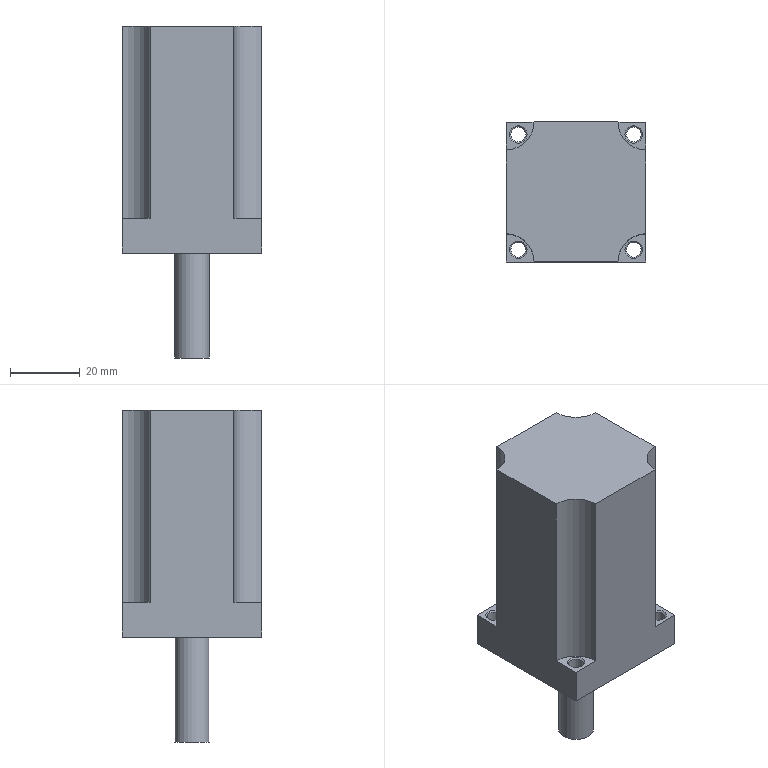Part | NX | features DATUM_CSYS 5, EXTRUDE 4, SIMPLE HOLE 4, SKETCH 4, SYMBOLIC_THREAD 4, HOLE PACKAGE 1 | 2 solids | 31 faces | box 40 x 40 x 95 mm | volume 97876 mm3 | plane 13 | cylinder 10 | cone 8 | commonest cylinder face diameters 4.2 x4 16 x4 10 x2
STEP:
#1=CARTESIAN_POINT('',(-14.,16.5,10.));
#2=VERTEX_POINT('',#1);
#3=CARTESIAN_POINT('',(-16.5,16.5,10.));
#4=DIRECTION('',(0.,0.,1.));
#5=DIRECTION('',(1.,0.,0.));
#6=AXIS2_PLACEMENT_3D('',#3,#4,#5);
#7=CIRCLE('',#6,2.5);
#8=EDGE_CURVE('',#2,#2,#7,.F.);
#9=ORIENTED_EDGE('',*,*,#8,.T.);
#10=EDGE_LOOP('',(#9));
#11=FACE_BOUND('',#10,.T.);
#12=CARTESIAN_POINT('',(-12.,20.,10.));
#13=VERTEX_POINT('',#12);
#14=CARTESIAN_POINT('',(-20.,12.,10.));
#15=VERTEX_POINT('',#14);
#16=CARTESIAN_POINT('',(-20.,20.,10.));
#17=DIRECTION('',(0.,0.,-1.));
#18=DIRECTION('',(0.,1.,0.));
#19=AXIS2_PLACEMENT_3D('',#16,#17,#18);
#20=CIRCLE('',#19,8.);
#21=EDGE_CURVE('',#13,#15,#20,.T.);
#22=ORIENTED_EDGE('',*,*,#21,.F.);
#23=CARTESIAN_POINT('',(-20.,20.,10.));
#24=VERTEX_POINT('',#23);
#25=CARTESIAN_POINT('',(20.,20.,10.));
#26=DIRECTION('',(-1.,0.,0.));
#27=VECTOR('',#26,1000.);
#28=LINE('',#25,#27);
#29=EDGE_CURVE('',#13,#24,#28,.T.);
#30=ORIENTED_EDGE('',*,*,#29,.T.);
#31=CARTESIAN_POINT('',(-20.,20.,10.));
#32=DIRECTION('',(0.,-1.,0.));
#33=VECTOR('',#32,1000.);
#34=LINE('',#31,#33);
#35=EDGE_CURVE('',#24,#15,#34,.T.);
#36=ORIENTED_EDGE('',*,*,#35,.T.);
#37=EDGE_LOOP('',(#22,#30,#36));
#38=FACE_BOUND('',#37,.T.);
#39=CARTESIAN_POINT('',(0.,0.,10.));
#40=DIRECTION('',(0.,0.,1.));
#41=DIRECTION('',(1.,0.,0.));
#42=AXIS2_PLACEMENT_3D('',#39,#40,#41);
#43=PLANE('',#42);
#44=ADVANCED_FACE('',(#11,#38),#43,.T.);
#45=CARTESIAN_POINT('',(19.,16.5,10.));
#46=VERTEX_POINT('',#45);
#47=CARTESIAN_POINT('',(16.5,16.5,10.));
#48=DIRECTION('',(0.,0.,1.));
#49=DIRECTION('',(1.,0.,0.));
#50=AXIS2_PLACEMENT_3D('',#47,#48,#49);
#51=CIRCLE('',#50,2.5);
#52=EDGE_CURVE('',#46,#46,#51,.F.);
#53=ORIENTED_EDGE('',*,*,#52,.T.);
#54=EDGE_LOOP('',(#53));
#55=FACE_BOUND('',#54,.T.);
#56=CARTESIAN_POINT('',(20.,12.,10.));
#57=VERTEX_POINT('',#56);
#58=CARTESIAN_POINT('',(12.,20.,10.));
#59=VERTEX_POINT('',#58);
#60=CARTESIAN_POINT('',(20.,20.,10.));
#61=DIRECTION('',(0.,0.,-1.));
#62=DIRECTION('',(0.,1.,0.));
#63=AXIS2_PLACEMENT_3D('',#60,#61,#62);
#64=CIRCLE('',#63,8.);
#65=EDGE_CURVE('',#57,#59,#64,.T.);
#66=ORIENTED_EDGE('',*,*,#65,.F.);
#67=CARTESIAN_POINT('',(20.,20.,10.));
#68=VERTEX_POINT('',#67);
#69=CARTESIAN_POINT('',(20.,-20.,10.));
#70=DIRECTION('',(0.,1.,0.));
#71=VECTOR('',#70,1000.);
#72=LINE('',#69,#71);
#73=EDGE_CURVE('',#57,#68,#72,.T.);
#74=ORIENTED_EDGE('',*,*,#73,.T.);
#75=CARTESIAN_POINT('',(20.,20.,10.));
#76=DIRECTION('',(-1.,0.,0.));
#77=VECTOR('',#76,1000.);
#78=LINE('',#75,#77);
#79=EDGE_CURVE('',#68,#59,#78,.T.);
#80=ORIENTED_EDGE('',*,*,#79,.T.);
#81=EDGE_LOOP('',(#66,#74,#80));
#82=FACE_BOUND('',#81,.T.);
#83=CARTESIAN_POINT('',(0.,0.,10.));
#84=DIRECTION('',(0.,0.,1.));
#85=DIRECTION('',(1.,0.,0.));
#86=AXIS2_PLACEMENT_3D('',#83,#84,#85);
#87=PLANE('',#86);
#88=ADVANCED_FACE('',(#55,#82),#87,.T.);
#89=CARTESIAN_POINT('',(19.,-16.5,10.));
#90=VERTEX_POINT('',#89);
#91=CARTESIAN_POINT('',(16.5,-16.5,10.));
#92=DIRECTION('',(0.,0.,1.));
#93=DIRECTION('',(1.,0.,0.));
#94=AXIS2_PLACEMENT_3D('',#91,#92,#93);
#95=CIRCLE('',#94,2.5);
#96=EDGE_CURVE('',#90,#90,#95,.F.);
#97=ORIENTED_EDGE('',*,*,#96,.T.);
#98=EDGE_LOOP('',(#97));
#99=FACE_BOUND('',#98,.T.);
#100=CARTESIAN_POINT('',(12.,-20.,10.));
#101=VERTEX_POINT('',#100);
#102=CARTESIAN_POINT('',(20.,-12.,10.));
#103=VERTEX_POINT('',#102);
#104=CARTESIAN_POINT('',(20.,-20.,10.));
#105=DIRECTION('',(0.,0.,-1.));
#106=DIRECTION('',(0.,-1.,0.));
#107=AXIS2_PLACEMENT_3D('',#104,#105,#106);
#108=CIRCLE('',#107,8.);
#109=EDGE_CURVE('',#101,#103,#108,.T.);
#110=ORIENTED_EDGE('',*,*,#109,.F.);
#111=CARTESIAN_POINT('',(20.,-20.,10.));
#112=VERTEX_POINT('',#111);
#113=CARTESIAN_POINT('',(-20.,-20.,10.));
#114=DIRECTION('',(1.,0.,0.));
#115=VECTOR('',#114,1000.);
#116=LINE('',#113,#115);
#117=EDGE_CURVE('',#101,#112,#116,.T.);
#118=ORIENTED_EDGE('',*,*,#117,.T.);
#119=CARTESIAN_POINT('',(20.,-20.,10.));
#120=DIRECTION('',(0.,1.,0.));
#121=VECTOR('',#120,1000.);
#122=LINE('',#119,#121);
#123=EDGE_CURVE('',#112,#103,#122,.T.);
#124=ORIENTED_EDGE('',*,*,#123,.T.);
#125=EDGE_LOOP('',(#110,#118,#124));
#126=FACE_BOUND('',#125,.T.);
#127=CARTESIAN_POINT('',(0.,0.,10.));
#128=DIRECTION('',(0.,0.,1.));
#129=DIRECTION('',(1.,0.,0.));
#130=AXIS2_PLACEMENT_3D('',#127,#128,#129);
#131=PLANE('',#130);
#132=ADVANCED_FACE('',(#99,#126),#131,.T.);
#133=CARTESIAN_POINT('',(-14.,-16.5,10.));
#134=VERTEX_POINT('',#133);
#135=CARTESIAN_POINT('',(-16.5,-16.5,10.));
#136=DIRECTION('',(0.,0.,1.));
#137=DIRECTION('',(1.,0.,0.));
#138=AXIS2_PLACEMENT_3D('',#135,#136,#137);
#139=CIRCLE('',#138,2.5);
#140=EDGE_CURVE('',#134,#134,#139,.F.);
#141=ORIENTED_EDGE('',*,*,#140,.T.);
#142=EDGE_LOOP('',(#141));
#143=FACE_BOUND('',#142,.T.);
#144=CARTESIAN_POINT('',(-20.,-12.,10.));
#145=VERTEX_POINT('',#144);
#146=CARTESIAN_POINT('',(-12.,-20.,10.));
#147=VERTEX_POINT('',#146);
#148=CARTESIAN_POINT('',(-20.,-20.,10.));
#149=DIRECTION('',(0.,0.,-1.));
#150=DIRECTION('',(0.,-1.,0.));
#151=AXIS2_PLACEMENT_3D('',#148,#149,#150);
#152=CIRCLE('',#151,8.);
#153=EDGE_CURVE('',#145,#147,#152,.T.);
#154=ORIENTED_EDGE('',*,*,#153,.F.);
#155=CARTESIAN_POINT('',(-20.,-20.,10.));
#156=VERTEX_POINT('',#155);
#157=CARTESIAN_POINT('',(-20.,20.,10.));
#158=DIRECTION('',(0.,-1.,0.));
#159=VECTOR('',#158,1000.);
#160=LINE('',#157,#159);
#161=EDGE_CURVE('',#145,#156,#160,.T.);
#162=ORIENTED_EDGE('',*,*,#161,.T.);
#163=CARTESIAN_POINT('',(-20.,-20.,10.));
#164=DIRECTION('',(1.,0.,0.));
#165=VECTOR('',#164,1000.);
#166=LINE('',#163,#165);
#167=EDGE_CURVE('',#156,#147,#166,.T.);
#168=ORIENTED_EDGE('',*,*,#167,.T.);
#169=EDGE_LOOP('',(#154,#162,#168));
#170=FACE_BOUND('',#169,.T.);
#171=CARTESIAN_POINT('',(0.,0.,10.));
#172=DIRECTION('',(0.,0.,1.));
#173=DIRECTION('',(1.,0.,0.));
#174=AXIS2_PLACEMENT_3D('',#171,#172,#173);
#175=PLANE('',#174);
#176=ADVANCED_FACE('',(#143,#170),#175,.T.);
#177=CARTESIAN_POINT('',(-20.,20.,0.));
#178=VERTEX_POINT('',#177);
#179=CARTESIAN_POINT('',(-20.,-20.,0.));
#180=VERTEX_POINT('',#179);
#181=CARTESIAN_POINT('',(-20.,20.,0.));
#182=DIRECTION('',(0.,-1.,0.));
#183=VECTOR('',#182,1000.);
#184=LINE('',#181,#183);
#185=EDGE_CURVE('',#178,#180,#184,.T.);
#186=ORIENTED_EDGE('',*,*,#185,.T.);
#187=CARTESIAN_POINT('',(-20.,-20.,10.));
#188=DIRECTION('',(0.,0.,-1.));
#189=VECTOR('',#188,1000.);
#190=LINE('',#187,#189);
#191=EDGE_CURVE('',#156,#180,#190,.T.);
#192=ORIENTED_EDGE('',*,*,#191,.F.);
#193=ORIENTED_EDGE('',*,*,#161,.F.);
#194=CARTESIAN_POINT('',(-20.,-12.,65.));
#195=VERTEX_POINT('',#194);
#196=CARTESIAN_POINT('',(-20.,-12.,65.));
#197=DIRECTION('',(0.,0.,-1.));
#198=VECTOR('',#197,1000.);
#199=LINE('',#196,#198);
#200=EDGE_CURVE('',#195,#145,#199,.T.);
#201=ORIENTED_EDGE('',*,*,#200,.F.);
#202=CARTESIAN_POINT('',(-20.,12.,65.));
#203=VERTEX_POINT('',#202);
#204=CARTESIAN_POINT('',(-20.,12.,65.));
#205=DIRECTION('',(0.,-1.,0.));
#206=VECTOR('',#205,1000.);
#207=LINE('',#204,#206);
#208=EDGE_CURVE('',#203,#195,#207,.T.);
#209=ORIENTED_EDGE('',*,*,#208,.F.);
#210=CARTESIAN_POINT('',(-20.,12.,65.));
#211=DIRECTION('',(0.,0.,-1.));
#212=VECTOR('',#211,1000.);
#213=LINE('',#210,#212);
#214=EDGE_CURVE('',#203,#15,#213,.T.);
#215=ORIENTED_EDGE('',*,*,#214,.T.);
#216=ORIENTED_EDGE('',*,*,#35,.F.);
#217=CARTESIAN_POINT('',(-20.,20.,10.));
#218=DIRECTION('',(0.,0.,-1.));
#219=VECTOR('',#218,1000.);
#220=LINE('',#217,#219);
#221=EDGE_CURVE('',#24,#178,#220,.T.);
#222=ORIENTED_EDGE('',*,*,#221,.T.);
#223=EDGE_LOOP('',(#186,#192,#193,#201,#209,#215,#216,#222));
#224=FACE_BOUND('',#223,.T.);
#225=CARTESIAN_POINT('',(-20.,20.,10.));
#226=DIRECTION('',(1.,0.,0.));
#227=DIRECTION('',(0.,0.,-1.));
#228=AXIS2_PLACEMENT_3D('',#225,#226,#227);
#229=PLANE('',#228);
#230=ADVANCED_FACE('',(#224),#229,.F.);
#231=CARTESIAN_POINT('',(20.,-20.,0.));
#232=VERTEX_POINT('',#231);
#233=CARTESIAN_POINT('',(-20.,-20.,0.));
#234=DIRECTION('',(1.,0.,0.));
#235=VECTOR('',#234,1000.);
#236=LINE('',#233,#235);
#237=EDGE_CURVE('',#180,#232,#236,.T.);
#238=ORIENTED_EDGE('',*,*,#237,.T.);
#239=CARTESIAN_POINT('',(20.,-20.,10.));
#240=DIRECTION('',(0.,0.,-1.));
#241=VECTOR('',#240,1000.);
#242=LINE('',#239,#241);
#243=EDGE_CURVE('',#112,#232,#242,.T.);
#244=ORIENTED_EDGE('',*,*,#243,.F.);
#245=ORIENTED_EDGE('',*,*,#117,.F.);
#246=CARTESIAN_POINT('',(12.,-20.,65.));
#247=VERTEX_POINT('',#246);
#248=CARTESIAN_POINT('',(12.,-20.,65.));
#249=DIRECTION('',(0.,0.,-1.));
#250=VECTOR('',#249,1000.);
#251=LINE('',#248,#250);
#252=EDGE_CURVE('',#247,#101,#251,.T.);
#253=ORIENTED_EDGE('',*,*,#252,.F.);
#254=CARTESIAN_POINT('',(-12.,-20.,65.));
#255=VERTEX_POINT('',#254);
#256=CARTESIAN_POINT('',(-12.,-20.,65.));
#257=DIRECTION('',(1.,0.,0.));
#258=VECTOR('',#257,1000.);
#259=LINE('',#256,#258);
#260=EDGE_CURVE('',#255,#247,#259,.T.);
#261=ORIENTED_EDGE('',*,*,#260,.F.);
#262=CARTESIAN_POINT('',(-12.,-20.,65.));
#263=DIRECTION('',(0.,0.,-1.));
#264=VECTOR('',#263,1000.);
#265=LINE('',#262,#264);
#266=EDGE_CURVE('',#255,#147,#265,.T.);
#267=ORIENTED_EDGE('',*,*,#266,.T.);
#268=ORIENTED_EDGE('',*,*,#167,.F.);
#269=ORIENTED_EDGE('',*,*,#191,.T.);
#270=EDGE_LOOP('',(#238,#244,#245,#253,#261,#267,#268,#269));
#271=FACE_BOUND('',#270,.T.);
#272=CARTESIAN_POINT('',(-20.,-20.,10.));
#273=DIRECTION('',(0.,1.,0.));
#274=DIRECTION('',(0.,0.,1.));
#275=AXIS2_PLACEMENT_3D('',#272,#273,#274);
#276=PLANE('',#275);
#277=ADVANCED_FACE('',(#271),#276,.F.);
#278=CARTESIAN_POINT('',(20.,20.,0.));
#279=VERTEX_POINT('',#278);
#280=CARTESIAN_POINT('',(20.,-20.,0.));
#281=DIRECTION('',(0.,1.,0.));
#282=VECTOR('',#281,1000.);
#283=LINE('',#280,#282);
#284=EDGE_CURVE('',#232,#279,#283,.T.);
#285=ORIENTED_EDGE('',*,*,#284,.T.);
#286=CARTESIAN_POINT('',(20.,20.,10.));
#287=DIRECTION('',(0.,0.,-1.));
#288=VECTOR('',#287,1000.);
#289=LINE('',#286,#288);
#290=EDGE_CURVE('',#68,#279,#289,.T.);
#291=ORIENTED_EDGE('',*,*,#290,.F.);
#292=ORIENTED_EDGE('',*,*,#73,.F.);
#293=CARTESIAN_POINT('',(20.,12.,65.));
#294=VERTEX_POINT('',#293);
#295=CARTESIAN_POINT('',(20.,12.,65.));
#296=DIRECTION('',(0.,0.,-1.));
#297=VECTOR('',#296,1000.);
#298=LINE('',#295,#297);
#299=EDGE_CURVE('',#294,#57,#298,.T.);
#300=ORIENTED_EDGE('',*,*,#299,.F.);
#301=CARTESIAN_POINT('',(20.,-12.,65.));
#302=VERTEX_POINT('',#301);
#303=CARTESIAN_POINT('',(20.,-12.,65.));
#304=DIRECTION('',(0.,1.,0.));
#305=VECTOR('',#304,1000.);
#306=LINE('',#303,#305);
#307=EDGE_CURVE('',#302,#294,#306,.T.);
#308=ORIENTED_EDGE('',*,*,#307,.F.);
#309=CARTESIAN_POINT('',(20.,-12.,65.));
#310=DIRECTION('',(0.,0.,-1.));
#311=VECTOR('',#310,1000.);
#312=LINE('',#309,#311);
#313=EDGE_CURVE('',#302,#103,#312,.T.);
#314=ORIENTED_EDGE('',*,*,#313,.T.);
#315=ORIENTED_EDGE('',*,*,#123,.F.);
#316=ORIENTED_EDGE('',*,*,#243,.T.);
#317=EDGE_LOOP('',(#285,#291,#292,#300,#308,#314,#315,#316));
#318=FACE_BOUND('',#317,.T.);
#319=CARTESIAN_POINT('',(20.,-20.,10.));
#320=DIRECTION('',(-1.,0.,0.));
#321=DIRECTION('',(0.,0.,1.));
#322=AXIS2_PLACEMENT_3D('',#319,#320,#321);
#323=PLANE('',#322);
#324=ADVANCED_FACE('',(#318),#323,.F.);
#325=CARTESIAN_POINT('',(20.,20.,0.));
#326=DIRECTION('',(-1.,0.,0.));
#327=VECTOR('',#326,1000.);
#328=LINE('',#325,#327);
#329=EDGE_CURVE('',#279,#178,#328,.T.);
#330=ORIENTED_EDGE('',*,*,#329,.T.);
#331=ORIENTED_EDGE('',*,*,#221,.F.);
#332=ORIENTED_EDGE('',*,*,#29,.F.);
#333=CARTESIAN_POINT('',(-12.,20.,65.));
#334=VERTEX_POINT('',#333);
#335=CARTESIAN_POINT('',(-12.,20.,65.));
#336=DIRECTION('',(0.,0.,-1.));
#337=VECTOR('',#336,1000.);
#338=LINE('',#335,#337);
#339=EDGE_CURVE('',#334,#13,#338,.T.);
#340=ORIENTED_EDGE('',*,*,#339,.F.);
#341=CARTESIAN_POINT('',(12.,20.,65.));
#342=VERTEX_POINT('',#341);
#343=CARTESIAN_POINT('',(12.,20.,65.));
#344=DIRECTION('',(-1.,0.,0.));
#345=VECTOR('',#344,1000.);
#346=LINE('',#343,#345);
#347=EDGE_CURVE('',#342,#334,#346,.T.);
#348=ORIENTED_EDGE('',*,*,#347,.F.);
#349=CARTESIAN_POINT('',(12.,20.,65.));
#350=DIRECTION('',(0.,0.,-1.));
#351=VECTOR('',#350,1000.);
#352=LINE('',#349,#351);
#353=EDGE_CURVE('',#342,#59,#352,.T.);
#354=ORIENTED_EDGE('',*,*,#353,.T.);
#355=ORIENTED_EDGE('',*,*,#79,.F.);
#356=ORIENTED_EDGE('',*,*,#290,.T.);
#357=EDGE_LOOP('',(#330,#331,#332,#340,#348,#354,#355,#356));
#358=FACE_BOUND('',#357,.T.);
#359=CARTESIAN_POINT('',(20.,20.,10.));
#360=DIRECTION('',(0.,-1.,0.));
#361=DIRECTION('',(0.,0.,-1.));
#362=AXIS2_PLACEMENT_3D('',#359,#360,#361);
#363=PLANE('',#362);
#364=ADVANCED_FACE('',(#358),#363,.F.);
#365=CARTESIAN_POINT('',(5.,0.,10.));
#366=VERTEX_POINT('',#365);
#367=CARTESIAN_POINT('',(0.,0.,10.));
#368=DIRECTION('',(0.,0.,1.));
#369=DIRECTION('',(1.,0.,0.));
#370=AXIS2_PLACEMENT_3D('',#367,#368,#369);
#371=CIRCLE('',#370,5.);
#372=EDGE_CURVE('',#366,#366,#371,.T.);
#373=ORIENTED_EDGE('',*,*,#372,.T.);
#374=EDGE_LOOP('',(#373));
#375=FACE_BOUND('',#374,.T.);
#376=CARTESIAN_POINT('',(5.,0.,0.));
#377=VERTEX_POINT('',#376);
#378=CARTESIAN_POINT('',(0.,0.,0.));
#379=DIRECTION('',(0.,0.,1.));
#380=DIRECTION('',(1.,0.,0.));
#381=AXIS2_PLACEMENT_3D('',#378,#379,#380);
#382=CIRCLE('',#381,5.);
#383=EDGE_CURVE('',#377,#377,#382,.T.);
#384=ORIENTED_EDGE('',*,*,#383,.F.);
#385=EDGE_LOOP('',(#384));
#386=FACE_BOUND('',#385,.T.);
#387=CARTESIAN_POINT('',(0.,0.,10.));
#388=DIRECTION('',(0.,0.,-1.));
#389=DIRECTION('',(-1.,0.,0.));
#390=AXIS2_PLACEMENT_3D('',#387,#388,#389);
#391=CYLINDRICAL_SURFACE('',#390,5.);
#392=ADVANCED_FACE('',(#375,#386),#391,.F.);
#393=CARTESIAN_POINT('',(19.,16.5,0.));
#394=VERTEX_POINT('',#393);
#395=CARTESIAN_POINT('',(16.5,16.5,0.));
#396=DIRECTION('',(0.,0.,1.));
#397=DIRECTION('',(1.,0.,0.));
#398=AXIS2_PLACEMENT_3D('',#395,#396,#397);
#399=CIRCLE('',#398,2.5);
#400=EDGE_CURVE('',#394,#394,#399,.T.);
#401=ORIENTED_EDGE('',*,*,#400,.T.);
#402=EDGE_LOOP('',(#401));
#403=FACE_BOUND('',#402,.T.);
#404=CARTESIAN_POINT('',(19.,-16.5,0.));
#405=VERTEX_POINT('',#404);
#406=CARTESIAN_POINT('',(16.5,-16.5,0.));
#407=DIRECTION('',(0.,0.,1.));
#408=DIRECTION('',(1.,0.,0.));
#409=AXIS2_PLACEMENT_3D('',#406,#407,#408);
#410=CIRCLE('',#409,2.5);
#411=EDGE_CURVE('',#405,#405,#410,.T.);
#412=ORIENTED_EDGE('',*,*,#411,.T.);
#413=EDGE_LOOP('',(#412));
#414=FACE_BOUND('',#413,.T.);
#415=CARTESIAN_POINT('',(-14.,16.5,0.));
#416=VERTEX_POINT('',#415);
#417=CARTESIAN_POINT('',(-16.5,16.5,0.));
#418=DIRECTION('',(0.,0.,1.));
#419=DIRECTION('',(1.,0.,0.));
#420=AXIS2_PLACEMENT_3D('',#417,#418,#419);
#421=CIRCLE('',#420,2.5);
#422=EDGE_CURVE('',#416,#416,#421,.T.);
#423=ORIENTED_EDGE('',*,*,#422,.T.);
#424=EDGE_LOOP('',(#423));
#425=FACE_BOUND('',#424,.T.);
#426=CARTESIAN_POINT('',(-14.,-16.5,0.));
#427=VERTEX_POINT('',#426);
#428=CARTESIAN_POINT('',(-16.5,-16.5,0.));
#429=DIRECTION('',(0.,0.,1.));
#430=DIRECTION('',(1.,0.,0.));
#431=AXIS2_PLACEMENT_3D('',#428,#429,#430);
#432=CIRCLE('',#431,2.5);
#433=EDGE_CURVE('',#427,#427,#432,.T.);
#434=ORIENTED_EDGE('',*,*,#433,.T.);
#435=EDGE_LOOP('',(#434));
#436=FACE_BOUND('',#435,.T.);
#437=ORIENTED_EDGE('',*,*,#185,.F.);
#438=ORIENTED_EDGE('',*,*,#329,.F.);
#439=ORIENTED_EDGE('',*,*,#284,.F.);
#440=ORIENTED_EDGE('',*,*,#237,.F.);
#441=EDGE_LOOP('',(#437,#438,#439,#440));
#442=FACE_BOUND('',#441,.T.);
#443=ORIENTED_EDGE('',*,*,#383,.T.);
#444=EDGE_LOOP('',(#443));
#445=FACE_BOUND('',#444,.T.);
#446=CARTESIAN_POINT('',(0.,0.,0.));
#447=DIRECTION('',(0.,0.,1.));
#448=DIRECTION('',(1.,0.,0.));
#449=AXIS2_PLACEMENT_3D('',#446,#447,#448);
#450=PLANE('',#449);
#451=ADVANCED_FACE('',(#403,#414,#425,#436,#442,#445),#450,.F.);
#452=ORIENTED_EDGE('',*,*,#208,.T.);
#453=CARTESIAN_POINT('',(-20.,-20.,65.));
#454=DIRECTION('',(0.,0.,-1.));
#455=DIRECTION('',(0.,-1.,0.));
#456=AXIS2_PLACEMENT_3D('',#453,#454,#455);
#457=CIRCLE('',#456,8.);
#458=EDGE_CURVE('',#195,#255,#457,.T.);
#459=ORIENTED_EDGE('',*,*,#458,.T.);
#460=ORIENTED_EDGE('',*,*,#260,.T.);
#461=CARTESIAN_POINT('',(20.,-20.,65.));
#462=DIRECTION('',(0.,0.,-1.));
#463=DIRECTION('',(0.,-1.,0.));
#464=AXIS2_PLACEMENT_3D('',#461,#462,#463);
#465=CIRCLE('',#464,8.);
#466=EDGE_CURVE('',#247,#302,#465,.T.);
#467=ORIENTED_EDGE('',*,*,#466,.T.);
#468=ORIENTED_EDGE('',*,*,#307,.T.);
#469=CARTESIAN_POINT('',(20.,20.,65.));
#470=DIRECTION('',(0.,0.,-1.));
#471=DIRECTION('',(0.,1.,0.));
#472=AXIS2_PLACEMENT_3D('',#469,#470,#471);
#473=CIRCLE('',#472,8.);
#474=EDGE_CURVE('',#294,#342,#473,.T.);
#475=ORIENTED_EDGE('',*,*,#474,.T.);
#476=ORIENTED_EDGE('',*,*,#347,.T.);
#477=CARTESIAN_POINT('',(-20.,20.,65.));
#478=DIRECTION('',(0.,0.,-1.));
#479=DIRECTION('',(0.,1.,0.));
#480=AXIS2_PLACEMENT_3D('',#477,#478,#479);
#481=CIRCLE('',#480,8.);
#482=EDGE_CURVE('',#334,#203,#481,.T.);
#483=ORIENTED_EDGE('',*,*,#482,.T.);
#484=EDGE_LOOP('',(#452,#459,#460,#467,#468,#475,#476,#483));
#485=FACE_BOUND('',#484,.T.);
#486=CARTESIAN_POINT('',(-20.,-20.,65.));
#487=DIRECTION('',(0.,0.,-1.));
#488=DIRECTION('',(-1.,0.,0.));
#489=AXIS2_PLACEMENT_3D('',#486,#487,#488);
#490=PLANE('',#489);
#491=ADVANCED_FACE('',(#485),#490,.F.);
#492=ORIENTED_EDGE('',*,*,#21,.T.);
#493=ORIENTED_EDGE('',*,*,#214,.F.);
#494=ORIENTED_EDGE('',*,*,#482,.F.);
#495=ORIENTED_EDGE('',*,*,#339,.T.);
#496=EDGE_LOOP('',(#492,#493,#494,#495));
#497=FACE_BOUND('',#496,.T.);
#498=CARTESIAN_POINT('',(-20.,20.,65.));
#499=DIRECTION('',(0.,0.,-1.));
#500=DIRECTION('',(-1.,0.,0.));
#501=AXIS2_PLACEMENT_3D('',#498,#499,#500);
#502=CYLINDRICAL_SURFACE('',#501,8.);
#503=ADVANCED_FACE('',(#497),#502,.F.);
#504=ORIENTED_EDGE('',*,*,#65,.T.);
#505=ORIENTED_EDGE('',*,*,#353,.F.);
#506=ORIENTED_EDGE('',*,*,#474,.F.);
#507=ORIENTED_EDGE('',*,*,#299,.T.);
#508=EDGE_LOOP('',(#504,#505,#506,#507));
#509=FACE_BOUND('',#508,.T.);
#510=CARTESIAN_POINT('',(20.,20.,65.));
#511=DIRECTION('',(0.,0.,-1.));
#512=DIRECTION('',(-1.,0.,0.));
#513=AXIS2_PLACEMENT_3D('',#510,#511,#512);
#514=CYLINDRICAL_SURFACE('',#513,8.);
#515=ADVANCED_FACE('',(#509),#514,.F.);
#516=ORIENTED_EDGE('',*,*,#109,.T.);
#517=ORIENTED_EDGE('',*,*,#313,.F.);
#518=ORIENTED_EDGE('',*,*,#466,.F.);
#519=ORIENTED_EDGE('',*,*,#252,.T.);
#520=EDGE_LOOP('',(#516,#517,#518,#519));
#521=FACE_BOUND('',#520,.T.);
#522=CARTESIAN_POINT('',(20.,-20.,65.));
#523=DIRECTION('',(0.,0.,-1.));
#524=DIRECTION('',(-1.,0.,0.));
#525=AXIS2_PLACEMENT_3D('',#522,#523,#524);
#526=CYLINDRICAL_SURFACE('',#525,8.);
#527=ADVANCED_FACE('',(#521),#526,.F.);
#528=ORIENTED_EDGE('',*,*,#153,.T.);
#529=ORIENTED_EDGE('',*,*,#266,.F.);
#530=ORIENTED_EDGE('',*,*,#458,.F.);
#531=ORIENTED_EDGE('',*,*,#200,.T.);
#532=EDGE_LOOP('',(#528,#529,#530,#531));
#533=FACE_BOUND('',#532,.T.);
#534=CARTESIAN_POINT('',(-20.,-20.,65.));
#535=DIRECTION('',(0.,0.,-1.));
#536=DIRECTION('',(-1.,0.,0.));
#537=AXIS2_PLACEMENT_3D('',#534,#535,#536);
#538=CYLINDRICAL_SURFACE('',#537,8.);
#539=ADVANCED_FACE('',(#533),#538,.F.);
#540=ORIENTED_EDGE('',*,*,#372,.F.);
#541=EDGE_LOOP('',(#540));
#542=FACE_BOUND('',#541,.T.);
#543=CARTESIAN_POINT('',(-20.,-20.,10.));
#544=DIRECTION('',(0.,0.,-1.));
#545=DIRECTION('',(-1.,0.,0.));
#546=AXIS2_PLACEMENT_3D('',#543,#544,#545);
#547=PLANE('',#546);
#548=ADVANCED_FACE('',(#542),#547,.T.);
#549=CARTESIAN_POINT('',(-14.4,-16.5,9.6));
#550=VERTEX_POINT('',#549);
#551=CARTESIAN_POINT('',(-16.5,-16.5,9.6));
#552=DIRECTION('',(0.,0.,1.));
#553=DIRECTION('',(1.,0.,0.));
#554=AXIS2_PLACEMENT_3D('',#551,#552,#553);
#555=CIRCLE('',#554,2.1);
#556=EDGE_CURVE('',#550,#550,#555,.T.);
#557=ORIENTED_EDGE('',*,*,#556,.T.);
#558=EDGE_LOOP('',(#557));
#559=FACE_BOUND('',#558,.T.);
#560=CARTESIAN_POINT('',(-14.4,-16.5,0.4));
#561=VERTEX_POINT('',#560);
#562=CARTESIAN_POINT('',(-16.5,-16.5,0.4));
#563=DIRECTION('',(0.,0.,1.));
#564=DIRECTION('',(1.,0.,0.));
#565=AXIS2_PLACEMENT_3D('',#562,#563,#564);
#566=CIRCLE('',#565,2.1);
#567=EDGE_CURVE('',#561,#561,#566,.F.);
#568=ORIENTED_EDGE('',*,*,#567,.T.);
#569=EDGE_LOOP('',(#568));
#570=FACE_BOUND('',#569,.T.);
#571=CARTESIAN_POINT('',(-16.5,-16.5,0.));
#572=DIRECTION('',(0.,0.,1.));
#573=DIRECTION('',(1.,0.,0.));
#574=AXIS2_PLACEMENT_3D('',#571,#572,#573);
#575=CYLINDRICAL_SURFACE('',#574,2.1);
#576=ADVANCED_FACE('',(#559,#570),#575,.F.);
#577=ORIENTED_EDGE('',*,*,#567,.F.);
#578=EDGE_LOOP('',(#577));
#579=FACE_BOUND('',#578,.T.);
#580=ORIENTED_EDGE('',*,*,#433,.F.);
#581=EDGE_LOOP('',(#580));
#582=FACE_BOUND('',#581,.T.);
#583=CARTESIAN_POINT('',(-16.5,-16.5,0.));
#584=DIRECTION('',(0.,0.,-1.));
#585=DIRECTION('',(-1.,0.,0.));
#586=AXIS2_PLACEMENT_3D('',#583,#584,#585);
#587=CONICAL_SURFACE('',#586,2.5,0.7854);
#588=ADVANCED_FACE('',(#579,#582),#587,.F.);
#589=ORIENTED_EDGE('',*,*,#140,.F.);
#590=EDGE_LOOP('',(#589));
#591=FACE_BOUND('',#590,.T.);
#592=ORIENTED_EDGE('',*,*,#556,.F.);
#593=EDGE_LOOP('',(#592));
#594=FACE_BOUND('',#593,.T.);
#595=CARTESIAN_POINT('',(-16.5,-16.5,9.6));
#596=DIRECTION('',(0.,0.,1.));
#597=DIRECTION('',(1.,0.,0.));
#598=AXIS2_PLACEMENT_3D('',#595,#596,#597);
#599=CONICAL_SURFACE('',#598,2.1,0.7854);
#600=ADVANCED_FACE('',(#591,#594),#599,.F.);
#601=CARTESIAN_POINT('',(-14.4,16.5,9.6));
#602=VERTEX_POINT('',#601);
#603=CARTESIAN_POINT('',(-16.5,16.5,9.6));
#604=DIRECTION('',(0.,0.,1.));
#605=DIRECTION('',(1.,0.,0.));
#606=AXIS2_PLACEMENT_3D('',#603,#604,#605);
#607=CIRCLE('',#606,2.1);
#608=EDGE_CURVE('',#602,#602,#607,.T.);
#609=ORIENTED_EDGE('',*,*,#608,.T.);
#610=EDGE_LOOP('',(#609));
#611=FACE_BOUND('',#610,.T.);
#612=CARTESIAN_POINT('',(-14.4,16.5,0.4));
#613=VERTEX_POINT('',#612);
#614=CARTESIAN_POINT('',(-16.5,16.5,0.4));
#615=DIRECTION('',(0.,0.,1.));
#616=DIRECTION('',(1.,0.,0.));
#617=AXIS2_PLACEMENT_3D('',#614,#615,#616);
#618=CIRCLE('',#617,2.1);
#619=EDGE_CURVE('',#613,#613,#618,.F.);
#620=ORIENTED_EDGE('',*,*,#619,.T.);
#621=EDGE_LOOP('',(#620));
#622=FACE_BOUND('',#621,.T.);
#623=CARTESIAN_POINT('',(-16.5,16.5,0.));
#624=DIRECTION('',(0.,0.,1.));
#625=DIRECTION('',(1.,0.,0.));
#626=AXIS2_PLACEMENT_3D('',#623,#624,#625);
#627=CYLINDRICAL_SURFACE('',#626,2.1);
#628=ADVANCED_FACE('',(#611,#622),#627,.F.);
#629=ORIENTED_EDGE('',*,*,#619,.F.);
#630=EDGE_LOOP('',(#629));
#631=FACE_BOUND('',#630,.T.);
#632=ORIENTED_EDGE('',*,*,#422,.F.);
#633=EDGE_LOOP('',(#632));
#634=FACE_BOUND('',#633,.T.);
#635=CARTESIAN_POINT('',(-16.5,16.5,0.));
#636=DIRECTION('',(0.,0.,-1.));
#637=DIRECTION('',(-1.,0.,0.));
#638=AXIS2_PLACEMENT_3D('',#635,#636,#637);
#639=CONICAL_SURFACE('',#638,2.5,0.7854);
#640=ADVANCED_FACE('',(#631,#634),#639,.F.);
#641=ORIENTED_EDGE('',*,*,#8,.F.);
#642=EDGE_LOOP('',(#641));
#643=FACE_BOUND('',#642,.T.);
#644=ORIENTED_EDGE('',*,*,#608,.F.);
#645=EDGE_LOOP('',(#644));
#646=FACE_BOUND('',#645,.T.);
#647=CARTESIAN_POINT('',(-16.5,16.5,9.6));
#648=DIRECTION('',(0.,0.,1.));
#649=DIRECTION('',(1.,0.,0.));
#650=AXIS2_PLACEMENT_3D('',#647,#648,#649);
#651=CONICAL_SURFACE('',#650,2.1,0.7854);
#652=ADVANCED_FACE('',(#643,#646),#651,.F.);
#653=CARTESIAN_POINT('',(18.6,-16.5,9.6));
#654=VERTEX_POINT('',#653);
#655=CARTESIAN_POINT('',(16.5,-16.5,9.6));
#656=DIRECTION('',(0.,0.,1.));
#657=DIRECTION('',(1.,0.,0.));
#658=AXIS2_PLACEMENT_3D('',#655,#656,#657);
#659=CIRCLE('',#658,2.1);
#660=EDGE_CURVE('',#654,#654,#659,.T.);
#661=ORIENTED_EDGE('',*,*,#660,.T.);
#662=EDGE_LOOP('',(#661));
#663=FACE_BOUND('',#662,.T.);
#664=CARTESIAN_POINT('',(18.6,-16.5,0.4));
#665=VERTEX_POINT('',#664);
#666=CARTESIAN_POINT('',(16.5,-16.5,0.4));
#667=DIRECTION('',(0.,0.,1.));
#668=DIRECTION('',(1.,0.,0.));
#669=AXIS2_PLACEMENT_3D('',#666,#667,#668);
#670=CIRCLE('',#669,2.1);
#671=EDGE_CURVE('',#665,#665,#670,.F.);
#672=ORIENTED_EDGE('',*,*,#671,.T.);
#673=EDGE_LOOP('',(#672));
#674=FACE_BOUND('',#673,.T.);
#675=CARTESIAN_POINT('',(16.5,-16.5,0.));
#676=DIRECTION('',(0.,0.,1.));
#677=DIRECTION('',(1.,0.,0.));
#678=AXIS2_PLACEMENT_3D('',#675,#676,#677);
#679=CYLINDRICAL_SURFACE('',#678,2.1);
#680=ADVANCED_FACE('',(#663,#674),#679,.F.);
#681=ORIENTED_EDGE('',*,*,#671,.F.);
#682=EDGE_LOOP('',(#681));
#683=FACE_BOUND('',#682,.T.);
#684=ORIENTED_EDGE('',*,*,#411,.F.);
#685=EDGE_LOOP('',(#684));
#686=FACE_BOUND('',#685,.T.);
#687=CARTESIAN_POINT('',(16.5,-16.5,0.));
#688=DIRECTION('',(0.,0.,-1.));
#689=DIRECTION('',(-1.,0.,0.));
#690=AXIS2_PLACEMENT_3D('',#687,#688,#689);
#691=CONICAL_SURFACE('',#690,2.5,0.7854);
#692=ADVANCED_FACE('',(#683,#686),#691,.F.);
#693=ORIENTED_EDGE('',*,*,#96,.F.);
#694=EDGE_LOOP('',(#693));
#695=FACE_BOUND('',#694,.T.);
#696=ORIENTED_EDGE('',*,*,#660,.F.);
#697=EDGE_LOOP('',(#696));
#698=FACE_BOUND('',#697,.T.);
#699=CARTESIAN_POINT('',(16.5,-16.5,9.6));
#700=DIRECTION('',(0.,0.,1.));
#701=DIRECTION('',(1.,0.,0.));
#702=AXIS2_PLACEMENT_3D('',#699,#700,#701);
#703=CONICAL_SURFACE('',#702,2.1,0.7854);
#704=ADVANCED_FACE('',(#695,#698),#703,.F.);
#705=CARTESIAN_POINT('',(18.6,16.5,9.6));
#706=VERTEX_POINT('',#705);
#707=CARTESIAN_POINT('',(16.5,16.5,9.6));
#708=DIRECTION('',(0.,0.,1.));
#709=DIRECTION('',(1.,0.,0.));
#710=AXIS2_PLACEMENT_3D('',#707,#708,#709);
#711=CIRCLE('',#710,2.1);
#712=EDGE_CURVE('',#706,#706,#711,.T.);
#713=ORIENTED_EDGE('',*,*,#712,.T.);
#714=EDGE_LOOP('',(#713));
#715=FACE_BOUND('',#714,.T.);
#716=CARTESIAN_POINT('',(18.6,16.5,0.4));
#717=VERTEX_POINT('',#716);
#718=CARTESIAN_POINT('',(16.5,16.5,0.4));
#719=DIRECTION('',(0.,0.,1.));
#720=DIRECTION('',(1.,0.,0.));
#721=AXIS2_PLACEMENT_3D('',#718,#719,#720);
#722=CIRCLE('',#721,2.1);
#723=EDGE_CURVE('',#717,#717,#722,.F.);
#724=ORIENTED_EDGE('',*,*,#723,.T.);
#725=EDGE_LOOP('',(#724));
#726=FACE_BOUND('',#725,.T.);
#727=CARTESIAN_POINT('',(16.5,16.5,0.));
#728=DIRECTION('',(0.,0.,1.));
#729=DIRECTION('',(1.,0.,0.));
#730=AXIS2_PLACEMENT_3D('',#727,#728,#729);
#731=CYLINDRICAL_SURFACE('',#730,2.1);
#732=ADVANCED_FACE('',(#715,#726),#731,.F.);
#733=ORIENTED_EDGE('',*,*,#723,.F.);
#734=EDGE_LOOP('',(#733));
#735=FACE_BOUND('',#734,.T.);
#736=ORIENTED_EDGE('',*,*,#400,.F.);
#737=EDGE_LOOP('',(#736));
#738=FACE_BOUND('',#737,.T.);
#739=CARTESIAN_POINT('',(16.5,16.5,0.));
#740=DIRECTION('',(0.,0.,-1.));
#741=DIRECTION('',(-1.,0.,0.));
#742=AXIS2_PLACEMENT_3D('',#739,#740,#741);
#743=CONICAL_SURFACE('',#742,2.5,0.7854);
#744=ADVANCED_FACE('',(#735,#738),#743,.F.);
#745=ORIENTED_EDGE('',*,*,#52,.F.);
#746=EDGE_LOOP('',(#745));
#747=FACE_BOUND('',#746,.T.);
#748=ORIENTED_EDGE('',*,*,#712,.F.);
#749=EDGE_LOOP('',(#748));
#750=FACE_BOUND('',#749,.T.);
#751=CARTESIAN_POINT('',(16.5,16.5,9.6));
#752=DIRECTION('',(0.,0.,1.));
#753=DIRECTION('',(1.,0.,0.));
#754=AXIS2_PLACEMENT_3D('',#751,#752,#753);
#755=CONICAL_SURFACE('',#754,2.1,0.7854);
#756=ADVANCED_FACE('',(#747,#750),#755,.F.);
#757=CLOSED_SHELL('',(#44,#88,#132,#176,#230,#277,#324,#364,#392,#451,#491,#503,#515,#527,#539,#548,#576,#588,#600,#628,#640,#652,#680,#692,#704,#732,#744,#756));
#758=MANIFOLD_SOLID_BREP('',#757);
#759=CARTESIAN_POINT('',(5.,0.,-30.));
#760=VERTEX_POINT('',#759);
#761=CARTESIAN_POINT('',(0.,0.,-30.));
#762=DIRECTION('',(0.,0.,1.));
#763=DIRECTION('',(1.,0.,0.));
#764=AXIS2_PLACEMENT_3D('',#761,#762,#763);
#765=CIRCLE('',#764,5.);
#766=EDGE_CURVE('',#760,#760,#765,.T.);
#767=ORIENTED_EDGE('',*,*,#766,.T.);
#768=EDGE_LOOP('',(#767));
#769=FACE_BOUND('',#768,.T.);
#770=CARTESIAN_POINT('',(5.,0.,50.));
#771=VERTEX_POINT('',#770);
#772=CARTESIAN_POINT('',(0.,0.,50.));
#773=DIRECTION('',(0.,0.,-1.));
#774=DIRECTION('',(1.,0.,0.));
#775=AXIS2_PLACEMENT_3D('',#772,#773,#774);
#776=CIRCLE('',#775,5.);
#777=EDGE_CURVE('',#771,#771,#776,.T.);
#778=ORIENTED_EDGE('',*,*,#777,.T.);
#779=EDGE_LOOP('',(#778));
#780=FACE_BOUND('',#779,.T.);
#781=CARTESIAN_POINT('',(0.,0.,-30.));
#782=DIRECTION('',(0.,0.,1.));
#783=DIRECTION('',(1.,0.,0.));
#784=AXIS2_PLACEMENT_3D('',#781,#782,#783);
#785=CYLINDRICAL_SURFACE('',#784,5.);
#786=ADVANCED_FACE('',(#769,#780),#785,.T.);
#787=ORIENTED_EDGE('',*,*,#766,.F.);
#788=EDGE_LOOP('',(#787));
#789=FACE_BOUND('',#788,.T.);
#790=CARTESIAN_POINT('',(0.,0.,-30.));
#791=DIRECTION('',(0.,0.,1.));
#792=DIRECTION('',(1.,0.,0.));
#793=AXIS2_PLACEMENT_3D('',#790,#791,#792);
#794=PLANE('',#793);
#795=ADVANCED_FACE('',(#789),#794,.F.);
#796=ORIENTED_EDGE('',*,*,#777,.F.);
#797=EDGE_LOOP('',(#796));
#798=FACE_BOUND('',#797,.T.);
#799=CARTESIAN_POINT('',(0.,0.,50.));
#800=DIRECTION('',(0.,0.,-1.));
#801=DIRECTION('',(-1.,0.,0.));
#802=AXIS2_PLACEMENT_3D('',#799,#800,#801);
#803=PLANE('',#802);
#804=ADVANCED_FACE('',(#798),#803,.F.);
#805=CLOSED_SHELL('',(#786,#795,#804));
#806=MANIFOLD_SOLID_BREP('',#805);
#807=(LENGTH_UNIT()NAMED_UNIT(*)SI_UNIT(.MILLI.,.METRE.));
#808=UNCERTAINTY_MEASURE_WITH_UNIT(LENGTH_MEASURE(0.00001),#807,'','');
#809=(NAMED_UNIT(*)PLANE_ANGLE_UNIT()SI_UNIT($,.RADIAN.));
#810=(NAMED_UNIT(*)SI_UNIT($,.STERADIAN.)SOLID_ANGLE_UNIT());
#811=(GEOMETRIC_REPRESENTATION_CONTEXT(3)GLOBAL_UNCERTAINTY_ASSIGNED_CONTEXT((#808))GLOBAL_UNIT_ASSIGNED_CONTEXT((#807,#809,#810))REPRESENTATION_CONTEXT('',''));
#812=ADVANCED_BREP_SHAPE_REPRESENTATION('',(#758,#806),#811);